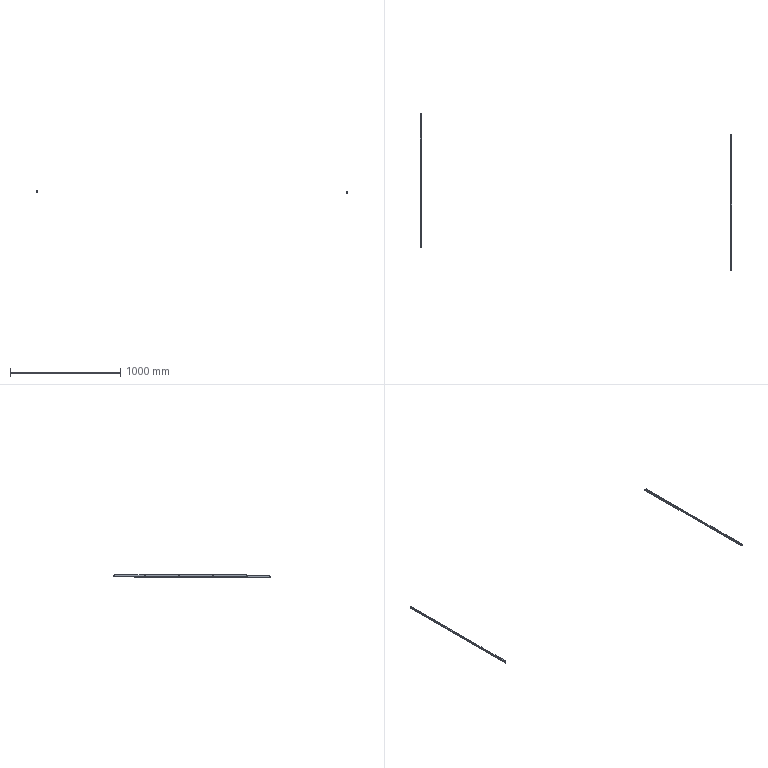NC program | NX | posted with a generic post | part box 2829 x 1430 x 20 mm
Whole program:
N10 G17 G21 G94 G90
(PLANAR_MILL_COPY_2 , TOOL : D16-48-D16-100-3T-FINISH)
N12 T01 M6
N14 G54
N16 G17 G0 G90 X633.5 Y-0.5 S4000 M3
N18 G43 Z30. H1
N20 Z2.
N22 G94 G1 Z0. F1000.
N24 X620.5
N26 X-620.5
N28 X-633.5
N30 Z2.
N32 G0 Z30.
N34 M5
(动态粗_COPY_1 , TOOL : D8-25-D8-60-3T-ROUGH)
N36 T02 M6
N38 G54
N40 G17 G0 G90 X619.561 Y-14.042 S6500 M3
N42 G43 Z30.2 H2
N44 Z-16.5
N46 G94 G1 X619.559 Y-14.017 Z-16.656 F3000.
N48 X619.557 Y-13.992 Z-16.718
N50 X619.555 Y-13.967 Z-16.763
N52 X619.552 Y-13.942 Z-16.8
N54 X619.55 Y-13.917 Z-16.831
N56 X619.548 Y-13.892 Z-16.857
N58 X619.546 Y-13.867 Z-16.88
N60 X619.544 Y-13.842 Z-16.9
N62 X619.542 Y-13.817 Z-16.918
N64 X619.539 Y-13.792 Z-16.933
N66 X619.537 Y-13.768 Z-16.947
N68 X619.535 Y-13.743 Z-16.958
N70 X619.533 Y-13.718 Z-16.968
N72 X619.531 Y-13.693 Z-16.977
N74 X619.529 Y-13.668 Z-16.984
N76 X619.526 Y-13.643 Z-16.99
N78 X619.524 Y-13.618 Z-16.994
N80 X619.522 Y-13.593 Z-16.997
N82 X619.52 Y-13.568 Z-16.999
N84 X619.518 Y-13.543 Z-17.
N86 X619.4 Y-12.186
N88 G3 X618.983 Y-11.547 R0.809
N90 X616.388 Y-10.819 R7.059
N92 X609.868 Y-10.524 R60.74
N94 G1 X599.395 Y-10.499
N96 X-618.005
N98 G2 X-620.945 Y-9.037 R4.184
N100 X-622.788 Y-5.306 R8.344
N102 X-623.386 Y-0.175 R26.77
N104 X-623.462 Y5.298 R95.282
N106 X-621.781 Y8.144 R4.438
N108 X-617.969 Y9.862 R8.929
N110 X-612.904 Y10.399 R29.555
N112 X-598.955 Y10.498 R480.604
N114 G1 X618.022
N116 G2 X621.01 Y8.974 R4.211
N118 X622.828 Y5.15 R8.583
N120 X623.397 Y-0.061 R28.776
N122 X623.463 Y-5.309 R102.326
N124 X621.736 Y-7.998 R3.791
N126 X618.162 Y-9.269 R8.341
N128 X613.148 Y-9.522 R36.711
N130 G1 X-613.527 Y-9.523
N132 G2 X-616.066 Y-9.452 R23.087
N134 X-617.171 Y-9.2 R30.278
N136 X-618.935 Y-9.095 R8.685
N138 G1 X-619.822 Y-8.784
N140 X-620.619 Y-8.284
N142 X-621.284 Y-7.619
N144 X-621.784 Y-6.822
N146 X-622.095 Y-5.935
N148 G2 X-622.2 Y-3.724 R12.124
N150 X-622.415 Y2.722 R92.718
N152 X-622.2 Y3.946 R10.556
N154 X-622.095 Y5.935 R9.581
N156 G1 X-621.784 Y6.822
N158 X-621.284 Y7.619
N160 X-620.619 Y8.284
N162 X-619.822 Y8.784
N164 X-618.935 Y9.095
N166 G2 X-616.649 Y9.2 R12.669
N168 X-603.589 Y9.492 R221.941
N170 G1 X-596.689 Y9.498
N172 X615.471 Y9.495
N174 G2 X617.091 Y9.207 R6.674
N176 X618.935 Y9.095 R9.79
N178 G1 X619.822 Y8.784
N180 X620.619 Y8.284
N182 X621.284 Y7.619
N184 X621.784 Y6.822
N186 X622.095 Y5.935
N188 G2 X622.2 Y3.724 R12.124
N190 X622.412 Y-2.542 R86.888
N192 X622.2 Y-3.673 R9.851
N194 X622.095 Y-5.935 R12.493
N196 G1 X621.784 Y-6.822
N198 X621.284 Y-7.619
N200 X620.619 Y-8.284
N202 X619.822 Y-8.784
N204 X618.935 Y-9.095
N206 X618. Y-9.2
N208 X-618.001
N210 X-618.935 Y-9.095
N212 X-619.822 Y-8.784
N214 X-620.619 Y-8.284
N216 X-621.284 Y-7.619
N218 X-621.784 Y-6.822
N220 X-622.095 Y-5.935
N222 G2 X-622.2 Y-3.724 R12.124
N224 G1 Y5.001
N226 X-622.095 Y5.935
N228 X-621.784 Y6.822
N230 X-621.284 Y7.619
N232 X-620.619 Y8.284
N234 X-619.822 Y8.784
N236 X-618.935 Y9.095
N238 G2 X-616.649 Y9.2 R12.669
N240 G1 X618.001
N242 X618.935 Y9.095
N244 X619.822 Y8.784
N246 X620.619 Y8.284
N248 X621.284 Y7.619
N250 X621.784 Y6.822
N252 X622.095 Y5.935
N254 G2 X622.2 Y3.724 R12.124
N256 G1 Y-3.701
N258 G3 X622.942 Y-4.506 R0.808
N260 G1 X624.156 Y-4.605
N262 X624.181 Y-4.607 Z-16.999
N264 X624.206 Y-4.609 Z-16.997
N266 X624.23 Y-4.611 Z-16.994
N268 X624.255 Y-4.613 Z-16.99
N270 X624.28 Y-4.615 Z-16.984
N272 X624.305 Y-4.617 Z-16.977
N274 X624.33 Y-4.619 Z-16.968
N276 X624.355 Y-4.621 Z-16.958
N278 X624.38 Y-4.624 Z-16.947
N280 X624.405 Y-4.626 Z-16.933
N282 X624.43 Y-4.628 Z-16.918
N284 X624.455 Y-4.63 Z-16.9
N286 X624.48 Y-4.632 Z-16.88
N288 X624.505 Y-4.634 Z-16.857
N290 X624.529 Y-4.636 Z-16.831
N292 X624.554 Y-4.638 Z-16.8
N294 X624.579 Y-4.64 Z-16.763
N296 X624.604 Y-4.642 Z-16.718
N298 X624.629 Y-4.644 Z-16.656
N300 X624.654 Y-4.646 Z-16.5
N302 G0 Z30.2
N304 M5
(PLANAR_MILL_1_COPY_2 , TOOL : D8-25-D8-60-3T-FINISH)
N306 T03 M6
N308 G54
N310 G17 G0 G90 X-624.928 Y9. S4500 M3
N312 G43 Z30. H3
N314 Z-15.
N316 G94 G1 Z-17. F1000.
N318 X-617.995
N320 X622.
N322 Y-9.
N324 X-622.
N326 Y4.995
N328 Y11.928
N330 Z-15.
N332 G0 Z30.
N334 X-624.928 Y9.
N336 Z-15.
N338 G1 Z-17.
N340 X-617.995
N342 X622.
N344 Y-9.
N346 X-622.
N348 Y4.995
N350 Y11.928
N352 Z-15.
N354 G0 Z30.
N356 M5
(PLANAR_MILL_1_COPY_COPY_1 , TOOL : 倒角D6-90度)
N358 T04 M6
N360 G54
N362 G17 G0 G90 X-619.5 Y-9.243 S4500 M3
N364 G43 Z30. H4
N366 Z0.5
N368 G94 G1 Z-1.5 F1000.
N370 Y-4.997
N372 Y6.5
N374 X619.5
N376 Y-6.5
N378 X-617.997
N380 X-622.243
N382 Z0.5
N384 G0 Z30.
N386 M5
N388 M2